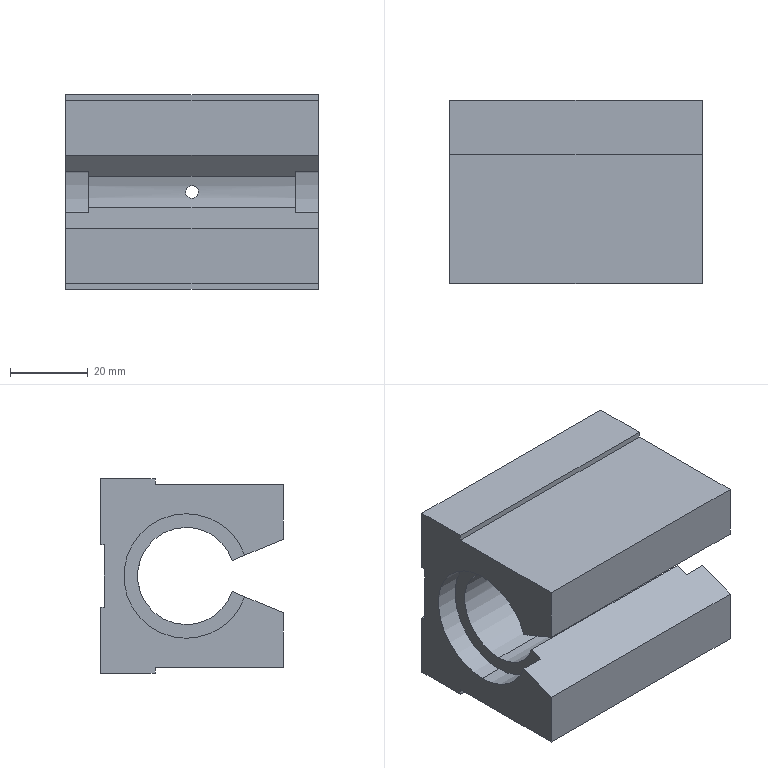Part | SolidWorks | features 3DProfileFeature 2, HoleWzd 2, ICE 2, Extrusion 1 | 1 solid | 46 faces | box 65 x 47 x 50 mm | volume 97950 mm3 | cylinder 19 | plane 19 | cone 8 | commonest cylinder face diameters 4.2 x8 32 x6 25 x3 3.3 x2
STEP:
#1=CARTESIAN_POINT('',(32.5,12.391,-1.65));
#2=VERTEX_POINT('',#1);
#3=CARTESIAN_POINT('',(32.5,12.391,1.65));
#4=VERTEX_POINT('',#3);
#5=CARTESIAN_POINT('',(32.5,12.391,-1.65));
#6=CARTESIAN_POINT('',(32.285,12.391,-1.65));
#7=CARTESIAN_POINT('',(32.067,12.397,-1.607));
#8=CARTESIAN_POINT('',(31.67,12.417,-1.442));
#9=CARTESIAN_POINT('',(31.486,12.431,-1.319));
#10=CARTESIAN_POINT('',(31.258,12.452,-1.092));
#11=CARTESIAN_POINT('',(31.188,12.46,-1.007));
#12=CARTESIAN_POINT('',(31.069,12.473,-0.8277));
#13=CARTESIAN_POINT('',(31.018,12.479,-0.733));
#14=CARTESIAN_POINT('',(30.935,12.489,-0.5333));
#15=CARTESIAN_POINT('',(30.903,12.493,-0.4285));
#16=CARTESIAN_POINT('',(30.861,12.499,-0.2176));
#17=CARTESIAN_POINT('',(30.85,12.5,-0.1102));
#18=CARTESIAN_POINT('',(30.85,12.5,0.1079));
#19=CARTESIAN_POINT('',(30.861,12.499,0.2152));
#20=CARTESIAN_POINT('',(30.902,12.493,0.4263));
#21=CARTESIAN_POINT('',(30.934,12.489,0.5312));
#22=CARTESIAN_POINT('',(31.017,12.479,0.7309));
#23=CARTESIAN_POINT('',(31.067,12.473,0.8257));
#24=CARTESIAN_POINT('',(31.187,12.46,1.005));
#25=CARTESIAN_POINT('',(31.257,12.453,1.09));
#26=CARTESIAN_POINT('',(31.484,12.431,1.318));
#27=CARTESIAN_POINT('',(31.668,12.417,1.441));
#28=CARTESIAN_POINT('',(32.065,12.397,1.606));
#29=CARTESIAN_POINT('',(32.282,12.391,1.65));
#30=CARTESIAN_POINT('',(32.5,12.391,1.65));
#31=B_SPLINE_CURVE_WITH_KNOTS('',3,(#5,#6,#7,#8,#9,#10,#11,#12,#13,#14,#15,#16,#17,#18,#19,#20,#21,#22,#23,#24,#25,#26,#27,#28,#29,#30),.UNSPECIFIED.,.F.,.F.,(4,2,2,2,2,2,2,2,2,2,2,2,4),(0.005164,0.00581,0.006455,0.006778,0.0071,0.007423,0.007746,0.008068,0.008391,0.008714,0.009037,0.009682,0.01033),.UNSPECIFIED.);
#32=EDGE_CURVE('',#2,#4,#31,.T.);
#33=ORIENTED_EDGE('',*,*,#32,.F.);
#34=CARTESIAN_POINT('',(32.5,21.,-1.65));
#35=VERTEX_POINT('',#34);
#36=CARTESIAN_POINT('',(32.5,22.,-1.65));
#37=DIRECTION('',(0.,1.,0.));
#38=VECTOR('',#37,1000.);
#39=LINE('',#36,#38);
#40=EDGE_CURVE('',#2,#35,#39,.T.);
#41=ORIENTED_EDGE('',*,*,#40,.T.);
#42=CARTESIAN_POINT('',(32.5,21.,1.65));
#43=VERTEX_POINT('',#42);
#44=CARTESIAN_POINT('',(32.5,21.,0.));
#45=DIRECTION('',(0.,-1.,0.));
#46=DIRECTION('',(0.,0.,-1.));
#47=AXIS2_PLACEMENT_3D('',#44,#45,#46);
#48=CIRCLE('',#47,1.65);
#49=EDGE_CURVE('',#43,#35,#48,.T.);
#50=ORIENTED_EDGE('',*,*,#49,.F.);
#51=CARTESIAN_POINT('',(32.5,22.,1.65));
#52=DIRECTION('',(0.,1.,0.));
#53=VECTOR('',#52,1000.);
#54=LINE('',#51,#53);
#55=EDGE_CURVE('',#4,#43,#54,.T.);
#56=ORIENTED_EDGE('',*,*,#55,.F.);
#57=EDGE_LOOP('',(#33,#41,#50,#56));
#58=FACE_OUTER_BOUND('',#57,.T.);
#59=CARTESIAN_POINT('',(32.5,22.,0.));
#60=DIRECTION('',(0.,1.,0.));
#61=DIRECTION('',(0.,0.,1.));
#62=AXIS2_PLACEMENT_3D('',#59,#60,#61);
#63=CYLINDRICAL_SURFACE('',#62,1.65);
#64=ADVANCED_FACE('',(#58),#63,.F.);
#65=CARTESIAN_POINT('',(12.5,9.6,-22.1));
#66=VERTEX_POINT('',#65);
#67=CARTESIAN_POINT('',(12.5,9.6,-17.9));
#68=VERTEX_POINT('',#67);
#69=CARTESIAN_POINT('',(12.5,9.6,-20.));
#70=DIRECTION('',(0.,1.,0.));
#71=DIRECTION('',(0.,0.,1.));
#72=AXIS2_PLACEMENT_3D('',#69,#70,#71);
#73=CIRCLE('',#72,2.1);
#74=EDGE_CURVE('',#66,#68,#73,.T.);
#75=ORIENTED_EDGE('',*,*,#74,.F.);
#76=CARTESIAN_POINT('',(12.5,22.,-22.1));
#77=VERTEX_POINT('',#76);
#78=CARTESIAN_POINT('',(12.5,22.,-22.1));
#79=DIRECTION('',(0.,1.,0.));
#80=VECTOR('',#79,1000.);
#81=LINE('',#78,#80);
#82=EDGE_CURVE('',#66,#77,#81,.T.);
#83=ORIENTED_EDGE('',*,*,#82,.T.);
#84=CARTESIAN_POINT('',(12.5,22.,-17.9));
#85=VERTEX_POINT('',#84);
#86=CARTESIAN_POINT('',(12.5,22.,-20.));
#87=DIRECTION('',(0.,1.,0.));
#88=DIRECTION('',(0.,0.,1.));
#89=AXIS2_PLACEMENT_3D('',#86,#87,#88);
#90=CIRCLE('',#89,2.1);
#91=EDGE_CURVE('',#77,#85,#90,.T.);
#92=ORIENTED_EDGE('',*,*,#91,.T.);
#93=CARTESIAN_POINT('',(12.5,22.,-17.9));
#94=DIRECTION('',(0.,1.,0.));
#95=VECTOR('',#94,1000.);
#96=LINE('',#93,#95);
#97=EDGE_CURVE('',#68,#85,#96,.T.);
#98=ORIENTED_EDGE('',*,*,#97,.F.);
#99=EDGE_LOOP('',(#75,#83,#92,#98));
#100=FACE_OUTER_BOUND('',#99,.T.);
#101=CARTESIAN_POINT('',(12.5,22.,-20.));
#102=DIRECTION('',(0.,1.,0.));
#103=DIRECTION('',(0.,0.,1.));
#104=AXIS2_PLACEMENT_3D('',#101,#102,#103);
#105=CYLINDRICAL_SURFACE('',#104,2.1);
#106=ADVANCED_FACE('',(#100),#105,.F.);
#107=CARTESIAN_POINT('',(12.5,8.338,-20.));
#108=VERTEX_POINT('',#107);
#109=CARTESIAN_POINT('',(12.5,9.6,-17.9));
#110=DIRECTION('',(0.,0.515,0.8572));
#111=VECTOR('',#110,1000.);
#112=LINE('',#109,#111);
#113=EDGE_CURVE('',#108,#68,#112,.T.);
#114=ORIENTED_EDGE('',*,*,#113,.F.);
#115=CARTESIAN_POINT('',(12.5,9.6,-22.1));
#116=DIRECTION('',(0.,0.515,-0.8572));
#117=VECTOR('',#116,1000.);
#118=LINE('',#115,#117);
#119=EDGE_CURVE('',#108,#66,#118,.T.);
#120=ORIENTED_EDGE('',*,*,#119,.T.);
#121=ORIENTED_EDGE('',*,*,#74,.T.);
#122=EDGE_LOOP('',(#114,#120,#121));
#123=FACE_OUTER_BOUND('',#122,.T.);
#124=CARTESIAN_POINT('',(12.5,9.6,-20.));
#125=DIRECTION('',(0.,1.,0.));
#126=DIRECTION('',(0.,0.,1.));
#127=AXIS2_PLACEMENT_3D('',#124,#125,#126);
#128=CONICAL_SURFACE('',#127,2.1,1.03);
#129=ADVANCED_FACE('',(#123),#128,.F.);
#130=CARTESIAN_POINT('',(52.5,9.6,-22.1));
#131=VERTEX_POINT('',#130);
#132=CARTESIAN_POINT('',(52.5,9.6,-17.9));
#133=VERTEX_POINT('',#132);
#134=CARTESIAN_POINT('',(52.5,9.6,-20.));
#135=DIRECTION('',(0.,1.,0.));
#136=DIRECTION('',(0.,0.,1.));
#137=AXIS2_PLACEMENT_3D('',#134,#135,#136);
#138=CIRCLE('',#137,2.1);
#139=EDGE_CURVE('',#131,#133,#138,.T.);
#140=ORIENTED_EDGE('',*,*,#139,.F.);
#141=CARTESIAN_POINT('',(52.5,22.,-22.1));
#142=VERTEX_POINT('',#141);
#143=CARTESIAN_POINT('',(52.5,22.,-22.1));
#144=DIRECTION('',(0.,1.,0.));
#145=VECTOR('',#144,1000.);
#146=LINE('',#143,#145);
#147=EDGE_CURVE('',#131,#142,#146,.T.);
#148=ORIENTED_EDGE('',*,*,#147,.T.);
#149=CARTESIAN_POINT('',(52.5,22.,-17.9));
#150=VERTEX_POINT('',#149);
#151=CARTESIAN_POINT('',(52.5,22.,-20.));
#152=DIRECTION('',(0.,1.,0.));
#153=DIRECTION('',(0.,0.,1.));
#154=AXIS2_PLACEMENT_3D('',#151,#152,#153);
#155=CIRCLE('',#154,2.1);
#156=EDGE_CURVE('',#142,#150,#155,.T.);
#157=ORIENTED_EDGE('',*,*,#156,.T.);
#158=CARTESIAN_POINT('',(52.5,22.,-17.9));
#159=DIRECTION('',(0.,1.,0.));
#160=VECTOR('',#159,1000.);
#161=LINE('',#158,#160);
#162=EDGE_CURVE('',#133,#150,#161,.T.);
#163=ORIENTED_EDGE('',*,*,#162,.F.);
#164=EDGE_LOOP('',(#140,#148,#157,#163));
#165=FACE_OUTER_BOUND('',#164,.T.);
#166=CARTESIAN_POINT('',(52.5,22.,-20.));
#167=DIRECTION('',(0.,1.,0.));
#168=DIRECTION('',(0.,0.,1.));
#169=AXIS2_PLACEMENT_3D('',#166,#167,#168);
#170=CYLINDRICAL_SURFACE('',#169,2.1);
#171=ADVANCED_FACE('',(#165),#170,.F.);
#172=CARTESIAN_POINT('',(52.5,8.338,-20.));
#173=VERTEX_POINT('',#172);
#174=CARTESIAN_POINT('',(52.5,9.6,-17.9));
#175=DIRECTION('',(0.,0.515,0.8572));
#176=VECTOR('',#175,1000.);
#177=LINE('',#174,#176);
#178=EDGE_CURVE('',#173,#133,#177,.T.);
#179=ORIENTED_EDGE('',*,*,#178,.F.);
#180=CARTESIAN_POINT('',(52.5,9.6,-22.1));
#181=DIRECTION('',(0.,0.515,-0.8572));
#182=VECTOR('',#181,1000.);
#183=LINE('',#180,#182);
#184=EDGE_CURVE('',#173,#131,#183,.T.);
#185=ORIENTED_EDGE('',*,*,#184,.T.);
#186=ORIENTED_EDGE('',*,*,#139,.T.);
#187=EDGE_LOOP('',(#179,#185,#186));
#188=FACE_OUTER_BOUND('',#187,.T.);
#189=CARTESIAN_POINT('',(52.5,9.6,-20.));
#190=DIRECTION('',(0.,1.,0.));
#191=DIRECTION('',(0.,0.,1.));
#192=AXIS2_PLACEMENT_3D('',#189,#190,#191);
#193=CONICAL_SURFACE('',#192,2.1,1.03);
#194=ADVANCED_FACE('',(#188),#193,.F.);
#195=CARTESIAN_POINT('',(12.5,9.6,17.9));
#196=VERTEX_POINT('',#195);
#197=CARTESIAN_POINT('',(12.5,9.6,22.1));
#198=VERTEX_POINT('',#197);
#199=CARTESIAN_POINT('',(12.5,9.6,20.));
#200=DIRECTION('',(0.,1.,0.));
#201=DIRECTION('',(0.,0.,1.));
#202=AXIS2_PLACEMENT_3D('',#199,#200,#201);
#203=CIRCLE('',#202,2.1);
#204=EDGE_CURVE('',#196,#198,#203,.T.);
#205=ORIENTED_EDGE('',*,*,#204,.F.);
#206=CARTESIAN_POINT('',(12.5,22.,17.9));
#207=VERTEX_POINT('',#206);
#208=CARTESIAN_POINT('',(12.5,22.,17.9));
#209=DIRECTION('',(0.,1.,0.));
#210=VECTOR('',#209,1000.);
#211=LINE('',#208,#210);
#212=EDGE_CURVE('',#196,#207,#211,.T.);
#213=ORIENTED_EDGE('',*,*,#212,.T.);
#214=CARTESIAN_POINT('',(12.5,22.,22.1));
#215=VERTEX_POINT('',#214);
#216=CARTESIAN_POINT('',(12.5,22.,20.));
#217=DIRECTION('',(0.,1.,0.));
#218=DIRECTION('',(0.,0.,1.));
#219=AXIS2_PLACEMENT_3D('',#216,#217,#218);
#220=CIRCLE('',#219,2.1);
#221=EDGE_CURVE('',#207,#215,#220,.T.);
#222=ORIENTED_EDGE('',*,*,#221,.T.);
#223=CARTESIAN_POINT('',(12.5,22.,22.1));
#224=DIRECTION('',(0.,1.,0.));
#225=VECTOR('',#224,1000.);
#226=LINE('',#223,#225);
#227=EDGE_CURVE('',#198,#215,#226,.T.);
#228=ORIENTED_EDGE('',*,*,#227,.F.);
#229=EDGE_LOOP('',(#205,#213,#222,#228));
#230=FACE_OUTER_BOUND('',#229,.T.);
#231=CARTESIAN_POINT('',(12.5,22.,20.));
#232=DIRECTION('',(0.,1.,0.));
#233=DIRECTION('',(0.,0.,1.));
#234=AXIS2_PLACEMENT_3D('',#231,#232,#233);
#235=CYLINDRICAL_SURFACE('',#234,2.1);
#236=ADVANCED_FACE('',(#230),#235,.F.);
#237=CARTESIAN_POINT('',(12.5,8.338,20.));
#238=VERTEX_POINT('',#237);
#239=CARTESIAN_POINT('',(12.5,9.6,22.1));
#240=DIRECTION('',(0.,0.515,0.8572));
#241=VECTOR('',#240,1000.);
#242=LINE('',#239,#241);
#243=EDGE_CURVE('',#238,#198,#242,.T.);
#244=ORIENTED_EDGE('',*,*,#243,.F.);
#245=CARTESIAN_POINT('',(12.5,9.6,17.9));
#246=DIRECTION('',(0.,0.515,-0.8572));
#247=VECTOR('',#246,1000.);
#248=LINE('',#245,#247);
#249=EDGE_CURVE('',#238,#196,#248,.T.);
#250=ORIENTED_EDGE('',*,*,#249,.T.);
#251=ORIENTED_EDGE('',*,*,#204,.T.);
#252=EDGE_LOOP('',(#244,#250,#251));
#253=FACE_OUTER_BOUND('',#252,.T.);
#254=CARTESIAN_POINT('',(12.5,9.6,20.));
#255=DIRECTION('',(0.,1.,0.));
#256=DIRECTION('',(0.,0.,1.));
#257=AXIS2_PLACEMENT_3D('',#254,#255,#256);
#258=CONICAL_SURFACE('',#257,2.1,1.03);
#259=ADVANCED_FACE('',(#253),#258,.F.);
#260=CARTESIAN_POINT('',(52.5,9.6,17.9));
#261=VERTEX_POINT('',#260);
#262=CARTESIAN_POINT('',(52.5,9.6,22.1));
#263=VERTEX_POINT('',#262);
#264=CARTESIAN_POINT('',(52.5,9.6,20.));
#265=DIRECTION('',(0.,1.,0.));
#266=DIRECTION('',(0.,0.,1.));
#267=AXIS2_PLACEMENT_3D('',#264,#265,#266);
#268=CIRCLE('',#267,2.1);
#269=EDGE_CURVE('',#261,#263,#268,.T.);
#270=ORIENTED_EDGE('',*,*,#269,.F.);
#271=CARTESIAN_POINT('',(52.5,22.,17.9));
#272=VERTEX_POINT('',#271);
#273=CARTESIAN_POINT('',(52.5,22.,17.9));
#274=DIRECTION('',(0.,1.,0.));
#275=VECTOR('',#274,1000.);
#276=LINE('',#273,#275);
#277=EDGE_CURVE('',#261,#272,#276,.T.);
#278=ORIENTED_EDGE('',*,*,#277,.T.);
#279=CARTESIAN_POINT('',(52.5,22.,22.1));
#280=VERTEX_POINT('',#279);
#281=CARTESIAN_POINT('',(52.5,22.,20.));
#282=DIRECTION('',(0.,1.,0.));
#283=DIRECTION('',(0.,0.,1.));
#284=AXIS2_PLACEMENT_3D('',#281,#282,#283);
#285=CIRCLE('',#284,2.1);
#286=EDGE_CURVE('',#272,#280,#285,.T.);
#287=ORIENTED_EDGE('',*,*,#286,.T.);
#288=CARTESIAN_POINT('',(52.5,22.,22.1));
#289=DIRECTION('',(0.,1.,0.));
#290=VECTOR('',#289,1000.);
#291=LINE('',#288,#290);
#292=EDGE_CURVE('',#263,#280,#291,.T.);
#293=ORIENTED_EDGE('',*,*,#292,.F.);
#294=EDGE_LOOP('',(#270,#278,#287,#293));
#295=FACE_OUTER_BOUND('',#294,.T.);
#296=CARTESIAN_POINT('',(52.5,22.,20.));
#297=DIRECTION('',(0.,1.,0.));
#298=DIRECTION('',(0.,0.,1.));
#299=AXIS2_PLACEMENT_3D('',#296,#297,#298);
#300=CYLINDRICAL_SURFACE('',#299,2.1);
#301=ADVANCED_FACE('',(#295),#300,.F.);
#302=CARTESIAN_POINT('',(52.5,8.338,20.));
#303=VERTEX_POINT('',#302);
#304=CARTESIAN_POINT('',(52.5,9.6,22.1));
#305=DIRECTION('',(0.,0.515,0.8572));
#306=VECTOR('',#305,1000.);
#307=LINE('',#304,#306);
#308=EDGE_CURVE('',#303,#263,#307,.T.);
#309=ORIENTED_EDGE('',*,*,#308,.F.);
#310=CARTESIAN_POINT('',(52.5,9.6,17.9));
#311=DIRECTION('',(0.,0.515,-0.8572));
#312=VECTOR('',#311,1000.);
#313=LINE('',#310,#312);
#314=EDGE_CURVE('',#303,#261,#313,.T.);
#315=ORIENTED_EDGE('',*,*,#314,.T.);
#316=ORIENTED_EDGE('',*,*,#269,.T.);
#317=EDGE_LOOP('',(#309,#315,#316));
#318=FACE_OUTER_BOUND('',#317,.T.);
#319=CARTESIAN_POINT('',(52.5,9.6,20.));
#320=DIRECTION('',(0.,1.,0.));
#321=DIRECTION('',(0.,0.,1.));
#322=AXIS2_PLACEMENT_3D('',#319,#320,#321);
#323=CONICAL_SURFACE('',#322,2.1,1.03);
#324=ADVANCED_FACE('',(#318),#323,.F.);
#325=CARTESIAN_POINT('',(6.,0.,-16.));
#326=VERTEX_POINT('',#325);
#327=CARTESIAN_POINT('',(6.,-15.082,-5.342));
#328=VERTEX_POINT('',#327);
#329=CARTESIAN_POINT('',(6.,0.,0.));
#330=DIRECTION('',(-1.,0.,0.));
#331=DIRECTION('',(0.,0.,1.));
#332=AXIS2_PLACEMENT_3D('',#329,#330,#331);
#333=CIRCLE('',#332,16.);
#334=EDGE_CURVE('',#326,#328,#333,.T.);
#335=ORIENTED_EDGE('',*,*,#334,.F.);
#336=CARTESIAN_POINT('',(0.,0.,-16.));
#337=VERTEX_POINT('',#336);
#338=CARTESIAN_POINT('',(6.,0.,-16.));
#339=DIRECTION('',(-1.,0.,0.));
#340=VECTOR('',#339,1000.);
#341=LINE('',#338,#340);
#342=EDGE_CURVE('',#326,#337,#341,.T.);
#343=ORIENTED_EDGE('',*,*,#342,.T.);
#344=CARTESIAN_POINT('',(0.,-15.082,-5.342));
#345=VERTEX_POINT('',#344);
#346=CARTESIAN_POINT('',(0.,0.,0.));
#347=DIRECTION('',(1.,0.,0.));
#348=DIRECTION('',(0.,0.,-1.));
#349=AXIS2_PLACEMENT_3D('',#346,#347,#348);
#350=CIRCLE('',#349,16.);
#351=EDGE_CURVE('',#345,#337,#350,.T.);
#352=ORIENTED_EDGE('',*,*,#351,.F.);
#353=CARTESIAN_POINT('',(6.,-15.082,-5.342));
#354=DIRECTION('',(-1.,0.,0.));
#355=VECTOR('',#354,1000.);
#356=LINE('',#353,#355);
#357=EDGE_CURVE('',#328,#345,#356,.T.);
#358=ORIENTED_EDGE('',*,*,#357,.F.);
#359=EDGE_LOOP('',(#335,#343,#352,#358));
#360=FACE_OUTER_BOUND('',#359,.T.);
#361=CARTESIAN_POINT('',(6.,0.,0.));
#362=DIRECTION('',(-1.,0.,0.));
#363=DIRECTION('',(0.,0.,1.));
#364=AXIS2_PLACEMENT_3D('',#361,#362,#363);
#365=CYLINDRICAL_SURFACE('',#364,16.);
#366=ADVANCED_FACE('',(#360),#365,.F.);
#367=ORIENTED_EDGE('',*,*,#342,.F.);
#368=CARTESIAN_POINT('',(6.,0.,16.));
#369=VERTEX_POINT('',#368);
#370=CARTESIAN_POINT('',(6.,0.,0.));
#371=DIRECTION('',(-1.,0.,0.));
#372=DIRECTION('',(0.,0.,1.));
#373=AXIS2_PLACEMENT_3D('',#370,#371,#372);
#374=CIRCLE('',#373,16.);
#375=EDGE_CURVE('',#369,#326,#374,.T.);
#376=ORIENTED_EDGE('',*,*,#375,.F.);
#377=CARTESIAN_POINT('',(0.,0.,16.));
#378=VERTEX_POINT('',#377);
#379=CARTESIAN_POINT('',(6.,0.,16.));
#380=DIRECTION('',(-1.,0.,0.));
#381=VECTOR('',#380,1000.);
#382=LINE('',#379,#381);
#383=EDGE_CURVE('',#369,#378,#382,.T.);
#384=ORIENTED_EDGE('',*,*,#383,.T.);
#385=CARTESIAN_POINT('',(0.,0.,0.));
#386=DIRECTION('',(1.,0.,0.));
#387=DIRECTION('',(0.,0.,-1.));
#388=AXIS2_PLACEMENT_3D('',#385,#386,#387);
#389=CIRCLE('',#388,16.);
#390=EDGE_CURVE('',#337,#378,#389,.T.);
#391=ORIENTED_EDGE('',*,*,#390,.F.);
#392=EDGE_LOOP('',(#367,#376,#384,#391));
#393=FACE_OUTER_BOUND('',#392,.T.);
#394=CARTESIAN_POINT('',(6.,0.,0.));
#395=DIRECTION('',(-1.,0.,0.));
#396=DIRECTION('',(0.,0.,1.));
#397=AXIS2_PLACEMENT_3D('',#394,#395,#396);
#398=CYLINDRICAL_SURFACE('',#397,16.);
#399=ADVANCED_FACE('',(#393),#398,.F.);
#400=CARTESIAN_POINT('',(59.,0.,16.));
#401=VERTEX_POINT('',#400);
#402=CARTESIAN_POINT('',(59.,-15.082,5.342));
#403=VERTEX_POINT('',#402);
#404=CARTESIAN_POINT('',(59.,0.,0.));
#405=DIRECTION('',(1.,0.,0.));
#406=DIRECTION('',(0.,0.,-1.));
#407=AXIS2_PLACEMENT_3D('',#404,#405,#406);
#408=CIRCLE('',#407,16.);
#409=EDGE_CURVE('',#401,#403,#408,.T.);
#410=ORIENTED_EDGE('',*,*,#409,.F.);
#411=CARTESIAN_POINT('',(65.,0.,16.));
#412=VERTEX_POINT('',#411);
#413=CARTESIAN_POINT('',(59.,0.,16.));
#414=DIRECTION('',(1.,0.,0.));
#415=VECTOR('',#414,1000.);
#416=LINE('',#413,#415);
#417=EDGE_CURVE('',#401,#412,#416,.T.);
#418=ORIENTED_EDGE('',*,*,#417,.T.);
#419=CARTESIAN_POINT('',(65.,-15.082,5.342));
#420=VERTEX_POINT('',#419);
#421=CARTESIAN_POINT('',(65.,0.,0.));
#422=DIRECTION('',(1.,0.,0.));
#423=DIRECTION('',(0.,0.,-1.));
#424=AXIS2_PLACEMENT_3D('',#421,#422,#423);
#425=CIRCLE('',#424,16.);
#426=EDGE_CURVE('',#412,#420,#425,.T.);
#427=ORIENTED_EDGE('',*,*,#426,.T.);
#428=CARTESIAN_POINT('',(59.,-15.082,5.342));
#429=DIRECTION('',(1.,0.,0.));
#430=VECTOR('',#429,1000.);
#431=LINE('',#428,#430);
#432=EDGE_CURVE('',#403,#420,#431,.T.);
#433=ORIENTED_EDGE('',*,*,#432,.F.);
#434=EDGE_LOOP('',(#410,#418,#427,#433));
#435=FACE_OUTER_BOUND('',#434,.T.);
#436=CARTESIAN_POINT('',(59.,0.,0.));
#437=DIRECTION('',(1.,0.,0.));
#438=DIRECTION('',(0.,0.,-1.));
#439=AXIS2_PLACEMENT_3D('',#436,#437,#438);
#440=CYLINDRICAL_SURFACE('',#439,16.);
#441=ADVANCED_FACE('',(#435),#440,.F.);
#442=ORIENTED_EDGE('',*,*,#417,.F.);
#443=CARTESIAN_POINT('',(59.,0.,-16.));
#444=VERTEX_POINT('',#443);
#445=CARTESIAN_POINT('',(59.,0.,0.));
#446=DIRECTION('',(1.,0.,0.));
#447=DIRECTION('',(0.,0.,-1.));
#448=AXIS2_PLACEMENT_3D('',#445,#446,#447);
#449=CIRCLE('',#448,16.);
#450=EDGE_CURVE('',#444,#401,#449,.T.);
#451=ORIENTED_EDGE('',*,*,#450,.F.);
#452=CARTESIAN_POINT('',(65.,0.,-16.));
#453=VERTEX_POINT('',#452);
#454=CARTESIAN_POINT('',(59.,0.,-16.));
#455=DIRECTION('',(1.,0.,0.));
#456=VECTOR('',#455,1000.);
#457=LINE('',#454,#456);
#458=EDGE_CURVE('',#444,#453,#457,.T.);
#459=ORIENTED_EDGE('',*,*,#458,.T.);
#460=CARTESIAN_POINT('',(65.,0.,0.));
#461=DIRECTION('',(1.,0.,0.));
#462=DIRECTION('',(0.,0.,-1.));
#463=AXIS2_PLACEMENT_3D('',#460,#461,#462);
#464=CIRCLE('',#463,16.);
#465=EDGE_CURVE('',#453,#412,#464,.T.);
#466=ORIENTED_EDGE('',*,*,#465,.T.);
#467=EDGE_LOOP('',(#442,#451,#459,#466));
#468=FACE_OUTER_BOUND('',#467,.T.);
#469=CARTESIAN_POINT('',(59.,0.,0.));
#470=DIRECTION('',(1.,0.,0.));
#471=DIRECTION('',(0.,0.,-1.));
#472=AXIS2_PLACEMENT_3D('',#469,#470,#471);
#473=CYLINDRICAL_SURFACE('',#472,16.);
#474=ADVANCED_FACE('',(#468),#473,.F.);
#475=CARTESIAN_POINT('',(59.,0.,-12.5));
#476=VERTEX_POINT('',#475);
#477=CARTESIAN_POINT('',(59.,-11.843,-4.));
#478=VERTEX_POINT('',#477);
#479=CARTESIAN_POINT('',(59.,0.,0.));
#480=DIRECTION('',(-1.,0.,0.));
#481=DIRECTION('',(0.,0.,-1.));
#482=AXIS2_PLACEMENT_3D('',#479,#480,#481);
#483=CIRCLE('',#482,12.5);
#484=EDGE_CURVE('',#476,#478,#483,.T.);
#485=ORIENTED_EDGE('',*,*,#484,.F.);
#486=CARTESIAN_POINT('',(6.,0.,-12.5));
#487=VERTEX_POINT('',#486);
#488=CARTESIAN_POINT('',(65.,0.,-12.5));
#489=DIRECTION('',(-1.,0.,0.));
#490=VECTOR('',#489,1000.);
#491=LINE('',#488,#490);
#492=EDGE_CURVE('',#476,#487,#491,.T.);
#493=ORIENTED_EDGE('',*,*,#492,.T.);
#494=CARTESIAN_POINT('',(6.,-11.843,-4.));
#495=VERTEX_POINT('',#494);
#496=CARTESIAN_POINT('',(6.,0.,0.));
#497=DIRECTION('',(1.,0.,0.));
#498=DIRECTION('',(0.,0.,1.));
#499=AXIS2_PLACEMENT_3D('',#496,#497,#498);
#500=CIRCLE('',#499,12.5);
#501=EDGE_CURVE('',#495,#487,#500,.T.);
#502=ORIENTED_EDGE('',*,*,#501,.F.);
#503=CARTESIAN_POINT('',(65.,-11.843,-4.));
#504=DIRECTION('',(-1.,0.,0.));
#505=VECTOR('',#504,1000.);
#506=LINE('',#503,#505);
#507=EDGE_CURVE('',#478,#495,#506,.T.);
#508=ORIENTED_EDGE('',*,*,#507,.F.);
#509=EDGE_LOOP('',(#485,#493,#502,#508));
#510=FACE_OUTER_BOUND('',#509,.T.);
#511=CARTESIAN_POINT('',(65.,0.,0.));
#512=DIRECTION('',(-1.,0.,0.));
#513=DIRECTION('',(0.,0.,1.));
#514=AXIS2_PLACEMENT_3D('',#511,#512,#513);
#515=CYLINDRICAL_SURFACE('',#514,12.5);
#516=ADVANCED_FACE('',(#510),#515,.F.);
#517=ORIENTED_EDGE('',*,*,#492,.F.);
#518=CARTESIAN_POINT('',(59.,0.,12.5));
#519=VERTEX_POINT('',#518);
#520=CARTESIAN_POINT('',(59.,0.,0.));
#521=DIRECTION('',(-1.,0.,0.));
#522=DIRECTION('',(0.,0.,-1.));
#523=AXIS2_PLACEMENT_3D('',#520,#521,#522);
#524=CIRCLE('',#523,12.5);
#525=EDGE_CURVE('',#519,#476,#524,.T.);
#526=ORIENTED_EDGE('',*,*,#525,.F.);
#527=CARTESIAN_POINT('',(6.,0.,12.5));
#528=VERTEX_POINT('',#527);
#529=CARTESIAN_POINT('',(65.,0.,12.5));
#530=DIRECTION('',(-1.,0.,0.));
#531=VECTOR('',#530,1000.);
#532=LINE('',#529,#531);
#533=EDGE_CURVE('',#519,#528,#532,.T.);
#534=ORIENTED_EDGE('',*,*,#533,.T.);
#535=CARTESIAN_POINT('',(6.,0.,0.));
#536=DIRECTION('',(1.,0.,0.));
#537=DIRECTION('',(0.,0.,1.));
#538=AXIS2_PLACEMENT_3D('',#535,#536,#537);
#539=CIRCLE('',#538,12.5);
#540=EDGE_CURVE('',#487,#528,#539,.T.);
#541=ORIENTED_EDGE('',*,*,#540,.F.);
#542=EDGE_LOOP('',(#517,#526,#534,#541));
#543=FACE_OUTER_BOUND('',#542,.T.);
#544=CARTESIAN_POINT('',(32.5,12.391,1.65));
#545=CARTESIAN_POINT('',(32.609,12.391,1.65));
#546=CARTESIAN_POINT('',(32.716,12.392,1.639));
#547=CARTESIAN_POINT('',(32.928,12.398,1.597));
#548=CARTESIAN_POINT('',(33.032,12.402,1.565));
#549=CARTESIAN_POINT('',(33.232,12.412,1.483));
#550=CARTESIAN_POINT('',(33.327,12.418,1.432));
#551=CARTESIAN_POINT('',(33.506,12.431,1.312));
#552=CARTESIAN_POINT('',(33.591,12.438,1.243));
#553=CARTESIAN_POINT('',(33.819,12.46,1.014));
#554=CARTESIAN_POINT('',(33.942,12.474,0.8305));
#555=CARTESIAN_POINT('',(34.106,12.494,0.4334));
#556=CARTESIAN_POINT('',(34.15,12.5,0.2161));
#557=CARTESIAN_POINT('',(34.15,12.5,-0.1071));
#558=CARTESIAN_POINT('',(34.139,12.499,-0.2166));
#559=CARTESIAN_POINT('',(34.097,12.493,-0.4283));
#560=CARTESIAN_POINT('',(34.066,12.489,-0.5312));
#561=CARTESIAN_POINT('',(33.983,12.479,-0.7312));
#562=CARTESIAN_POINT('',(33.931,12.473,-0.8276));
#563=CARTESIAN_POINT('',(33.812,12.46,-1.006));
#564=CARTESIAN_POINT('',(33.744,12.453,-1.09));
#565=CARTESIAN_POINT('',(33.59,12.438,-1.244));
#566=CARTESIAN_POINT('',(33.507,12.431,-1.312));
#567=CARTESIAN_POINT('',(33.328,12.418,-1.431));
#568=CARTESIAN_POINT('',(33.232,12.412,-1.483));
#569=CARTESIAN_POINT('',(33.032,12.402,-1.566));
#570=CARTESIAN_POINT('',(32.929,12.398,-1.597));
#571=CARTESIAN_POINT('',(32.717,12.392,-1.639));
#572=CARTESIAN_POINT('',(32.608,12.391,-1.65));
#573=CARTESIAN_POINT('',(32.5,12.391,-1.65));
#574=B_SPLINE_CURVE_WITH_KNOTS('',3,(#544,#545,#546,#547,#548,#549,#550,#551,#552,#553,#554,#555,#556,#557,#558,#559,#560,#561,#562,#563,#564,#565,#566,#567,#568,#569,#570,#571,#572,#573),.UNSPECIFIED.,.F.,.F.,(4,2,2,2,2,2,2,2,2,2,2,2,2,2,4),(0.,0.0003228,0.0006455,0.0009683,0.001291,0.001937,0.002582,0.002905,0.003228,0.00355,0.003873,0.004196,0.004519,0.004842,0.005164),.UNSPECIFIED.);
#575=EDGE_CURVE('',#4,#2,#574,.T.);
#576=ORIENTED_EDGE('',*,*,#575,.T.);
#577=ORIENTED_EDGE('',*,*,#32,.T.);
#578=EDGE_LOOP('',(#576,#577));
#579=FACE_BOUND('',#578,.T.);
#580=CARTESIAN_POINT('',(65.,0.,0.));
#581=DIRECTION('',(-1.,0.,0.));
#582=DIRECTION('',(0.,0.,1.));
#583=AXIS2_PLACEMENT_3D('',#580,#581,#582);
#584=CYLINDRICAL_SURFACE('',#583,12.5);
#585=ADVANCED_FACE('',(#543,#579),#584,.F.);
#586=ORIENTED_EDGE('',*,*,#533,.F.);
#587=CARTESIAN_POINT('',(59.,-11.843,4.));
#588=VERTEX_POINT('',#587);
#589=CARTESIAN_POINT('',(59.,0.,0.));
#590=DIRECTION('',(-1.,0.,0.));
#591=DIRECTION('',(0.,0.,-1.));
#592=AXIS2_PLACEMENT_3D('',#589,#590,#591);
#593=CIRCLE('',#592,12.5);
#594=EDGE_CURVE('',#588,#519,#593,.T.);
#595=ORIENTED_EDGE('',*,*,#594,.F.);
#596=CARTESIAN_POINT('',(6.,-11.843,4.));
#597=VERTEX_POINT('',#596);
#598=CARTESIAN_POINT('',(65.,-11.843,4.));
#599=DIRECTION('',(-1.,0.,0.));
#600=VECTOR('',#599,1000.);
#601=LINE('',#598,#600);
#602=EDGE_CURVE('',#588,#597,#601,.T.);
#603=ORIENTED_EDGE('',*,*,#602,.T.);
#604=CARTESIAN_POINT('',(6.,0.,0.));
#605=DIRECTION('',(1.,0.,0.));
#606=DIRECTION('',(0.,0.,1.));
#607=AXIS2_PLACEMENT_3D('',#604,#605,#606);
#608=CIRCLE('',#607,12.5);
#609=EDGE_CURVE('',#528,#597,#608,.T.);
#610=ORIENTED_EDGE('',*,*,#609,.F.);
#611=EDGE_LOOP('',(#586,#595,#603,#610));
#612=FACE_OUTER_BOUND('',#611,.T.);
#613=CARTESIAN_POINT('',(65.,0.,0.));
#614=DIRECTION('',(-1.,0.,0.));
#615=DIRECTION('',(0.,0.,1.));
#616=AXIS2_PLACEMENT_3D('',#613,#614,#615);
#617=CYLINDRICAL_SURFACE('',#616,12.5);
#618=ADVANCED_FACE('',(#612),#617,.F.);
#619=CARTESIAN_POINT('',(6.,-25.,-9.45));
#620=DIRECTION('',(0.,0.9239,0.3827));
#621=VECTOR('',#620,1000.);
#622=LINE('',#619,#621);
#623=EDGE_CURVE('',#328,#495,#622,.T.);
#624=ORIENTED_EDGE('',*,*,#623,.F.);
#625=ORIENTED_EDGE('',*,*,#357,.T.);
#626=CARTESIAN_POINT('',(0.,-25.,-9.45));
#627=VERTEX_POINT('',#626);
#628=CARTESIAN_POINT('',(0.,-25.,-9.45));
#629=DIRECTION('',(0.,-0.9239,-0.3827));
#630=VECTOR('',#629,1000.);
#631=LINE('',#628,#630);
#632=EDGE_CURVE('',#345,#627,#631,.T.);
#633=ORIENTED_EDGE('',*,*,#632,.T.);
#634=CARTESIAN_POINT('',(65.,-25.,-9.45));
#635=VERTEX_POINT('',#634);
#636=CARTESIAN_POINT('',(65.,-25.,-9.45));
#637=DIRECTION('',(-1.,0.,0.));
#638=VECTOR('',#637,1000.);
#639=LINE('',#636,#638);
#640=EDGE_CURVE('',#635,#627,#639,.T.);
#641=ORIENTED_EDGE('',*,*,#640,.F.);
#642=CARTESIAN_POINT('',(65.,-15.082,-5.342));
#643=VERTEX_POINT('',#642);
#644=CARTESIAN_POINT('',(65.,-25.,-9.45));
#645=DIRECTION('',(0.,-0.9239,-0.3827));
#646=VECTOR('',#645,1000.);
#647=LINE('',#644,#646);
#648=EDGE_CURVE('',#643,#635,#647,.T.);
#649=ORIENTED_EDGE('',*,*,#648,.F.);
#650=CARTESIAN_POINT('',(59.,-15.082,-5.342));
#651=VERTEX_POINT('',#650);
#652=CARTESIAN_POINT('',(59.,-15.082,-5.342));
#653=DIRECTION('',(-1.,0.,0.));
#654=VECTOR('',#653,1000.);
#655=LINE('',#652,#654);
#656=EDGE_CURVE('',#643,#651,#655,.T.);
#657=ORIENTED_EDGE('',*,*,#656,.T.);
#658=CARTESIAN_POINT('',(59.,-25.,-9.45));
#659=DIRECTION('',(0.,-0.9239,-0.3827));
#660=VECTOR('',#659,1000.);
#661=LINE('',#658,#660);
#662=EDGE_CURVE('',#478,#651,#661,.T.);
#663=ORIENTED_EDGE('',*,*,#662,.F.);
#664=ORIENTED_EDGE('',*,*,#507,.T.);
#665=EDGE_LOOP('',(#624,#625,#633,#641,#649,#657,#663,#664));
#666=FACE_OUTER_BOUND('',#665,.T.);
#667=CARTESIAN_POINT('',(65.,-25.,-9.45));
#668=DIRECTION('',(0.,0.3827,-0.9239));
#669=DIRECTION('',(0.,0.9239,0.3827));
#670=AXIS2_PLACEMENT_3D('',#667,#668,#669);
#671=PLANE('',#670);
#672=ADVANCED_FACE('',(#666),#671,.F.);
#673=CARTESIAN_POINT('',(0.,-25.,-23.5));
#674=VERTEX_POINT('',#673);
#675=CARTESIAN_POINT('',(0.,-25.,-9.45));
#676=DIRECTION('',(0.,0.,-1.));
#677=VECTOR('',#676,1000.);
#678=LINE('',#675,#677);
#679=EDGE_CURVE('',#627,#674,#678,.T.);
#680=ORIENTED_EDGE('',*,*,#679,.T.);
#681=CARTESIAN_POINT('',(65.,-25.,-23.5));
#682=VERTEX_POINT('',#681);
#683=CARTESIAN_POINT('',(65.,-25.,-23.5));
#684=DIRECTION('',(-1.,0.,0.));
#685=VECTOR('',#684,1000.);
#686=LINE('',#683,#685);
#687=EDGE_CURVE('',#682,#674,#686,.T.);
#688=ORIENTED_EDGE('',*,*,#687,.F.);
#689=CARTESIAN_POINT('',(65.,-25.,-9.45));
#690=DIRECTION('',(0.,0.,-1.));
#691=VECTOR('',#690,1000.);
#692=LINE('',#689,#691);
#693=EDGE_CURVE('',#635,#682,#692,.T.);
#694=ORIENTED_EDGE('',*,*,#693,.F.);
#695=ORIENTED_EDGE('',*,*,#640,.T.);
#696=EDGE_LOOP('',(#680,#688,#694,#695));
#697=FACE_OUTER_BOUND('',#696,.T.);
#698=CARTESIAN_POINT('',(65.,-25.,-9.45));
#699=DIRECTION('',(0.,1.,0.));
#700=DIRECTION('',(0.,0.,1.));
#701=AXIS2_PLACEMENT_3D('',#698,#699,#700);
#702=PLANE('',#701);
#703=ADVANCED_FACE('',(#697),#702,.F.);
#704=CARTESIAN_POINT('',(0.,8.,-23.5));
#705=VERTEX_POINT('',#704);
#706=CARTESIAN_POINT('',(0.,-25.,-23.5));
#707=DIRECTION('',(0.,1.,0.));
#708=VECTOR('',#707,1000.);
#709=LINE('',#706,#708);
#710=EDGE_CURVE('',#674,#705,#709,.T.);
#711=ORIENTED_EDGE('',*,*,#710,.T.);
#712=CARTESIAN_POINT('',(65.,8.,-23.5));
#713=VERTEX_POINT('',#712);
#714=CARTESIAN_POINT('',(65.,8.,-23.5));
#715=DIRECTION('',(-1.,0.,0.));
#716=VECTOR('',#715,1000.);
#717=LINE('',#714,#716);
#718=EDGE_CURVE('',#713,#705,#717,.T.);
#719=ORIENTED_EDGE('',*,*,#718,.F.);
#720=CARTESIAN_POINT('',(65.,-25.,-23.5));
#721=DIRECTION('',(0.,1.,0.));
#722=VECTOR('',#721,1000.);
#723=LINE('',#720,#722);
#724=EDGE_CURVE('',#682,#713,#723,.T.);
#725=ORIENTED_EDGE('',*,*,#724,.F.);
#726=ORIENTED_EDGE('',*,*,#687,.T.);
#727=EDGE_LOOP('',(#711,#719,#725,#726));
#728=FACE_OUTER_BOUND('',#727,.T.);
#729=CARTESIAN_POINT('',(65.,-25.,-23.5));
#730=DIRECTION('',(0.,0.,1.));
#731=DIRECTION('',(1.,0.,0.));
#732=AXIS2_PLACEMENT_3D('',#729,#730,#731);
#733=PLANE('',#732);
#734=ADVANCED_FACE('',(#728),#733,.F.);
#735=CARTESIAN_POINT('',(0.,8.,-25.));
#736=VERTEX_POINT('',#735);
#737=CARTESIAN_POINT('',(0.,8.,-23.5));
#738=DIRECTION('',(0.,0.,-1.));
#739=VECTOR('',#738,1000.);
#740=LINE('',#737,#739);
#741=EDGE_CURVE('',#705,#736,#740,.T.);
#742=ORIENTED_EDGE('',*,*,#741,.T.);
#743=CARTESIAN_POINT('',(65.,8.,-25.));
#744=VERTEX_POINT('',#743);
#745=CARTESIAN_POINT('',(65.,8.,-25.));
#746=DIRECTION('',(-1.,0.,0.));
#747=VECTOR('',#746,1000.);
#748=LINE('',#745,#747);
#749=EDGE_CURVE('',#744,#736,#748,.T.);
#750=ORIENTED_EDGE('',*,*,#749,.F.);
#751=CARTESIAN_POINT('',(65.,8.,-23.5));
#752=DIRECTION('',(0.,0.,-1.));
#753=VECTOR('',#752,1000.);
#754=LINE('',#751,#753);
#755=EDGE_CURVE('',#713,#744,#754,.T.);
#756=ORIENTED_EDGE('',*,*,#755,.F.);
#757=ORIENTED_EDGE('',*,*,#718,.T.);
#758=EDGE_LOOP('',(#742,#750,#756,#757));
#759=FACE_OUTER_BOUND('',#758,.T.);
#760=CARTESIAN_POINT('',(65.,8.,-23.5));
#761=DIRECTION('',(0.,1.,0.));
#762=DIRECTION('',(0.,0.,1.));
#763=AXIS2_PLACEMENT_3D('',#760,#761,#762);
#764=PLANE('',#763);
#765=ADVANCED_FACE('',(#759),#764,.F.);
#766=CARTESIAN_POINT('',(0.,22.,-25.));
#767=VERTEX_POINT('',#766);
#768=CARTESIAN_POINT('',(0.,8.,-25.));
#769=DIRECTION('',(0.,1.,0.));
#770=VECTOR('',#769,1000.);
#771=LINE('',#768,#770);
#772=EDGE_CURVE('',#736,#767,#771,.T.);
#773=ORIENTED_EDGE('',*,*,#772,.T.);
#774=CARTESIAN_POINT('',(65.,22.,-25.));
#775=VERTEX_POINT('',#774);
#776=CARTESIAN_POINT('',(65.,22.,-25.));
#777=DIRECTION('',(-1.,0.,0.));
#778=VECTOR('',#777,1000.);
#779=LINE('',#776,#778);
#780=EDGE_CURVE('',#775,#767,#779,.T.);
#781=ORIENTED_EDGE('',*,*,#780,.F.);
#782=CARTESIAN_POINT('',(65.,8.,-25.));
#783=DIRECTION('',(0.,1.,0.));
#784=VECTOR('',#783,1000.);
#785=LINE('',#782,#784);
#786=EDGE_CURVE('',#744,#775,#785,.T.);
#787=ORIENTED_EDGE('',*,*,#786,.F.);
#788=ORIENTED_EDGE('',*,*,#749,.T.);
#789=EDGE_LOOP('',(#773,#781,#787,#788));
#790=FACE_OUTER_BOUND('',#789,.T.);
#791=CARTESIAN_POINT('',(65.,8.,-25.));
#792=DIRECTION('',(0.,0.,1.));
#793=DIRECTION('',(1.,0.,0.));
#794=AXIS2_PLACEMENT_3D('',#791,#792,#793);
#795=PLANE('',#794);
#796=ADVANCED_FACE('',(#790),#795,.F.);
#797=CARTESIAN_POINT('',(12.5,22.,-20.));
#798=DIRECTION('',(0.,1.,0.));
#799=DIRECTION('',(0.,0.,1.));
#800=AXIS2_PLACEMENT_3D('',#797,#798,#799);
#801=CIRCLE('',#800,2.1);
#802=EDGE_CURVE('',#85,#77,#801,.T.);
#803=ORIENTED_EDGE('',*,*,#802,.F.);
#804=ORIENTED_EDGE('',*,*,#91,.F.);
#805=EDGE_LOOP('',(#803,#804));
#806=FACE_BOUND('',#805,.T.);
#807=CARTESIAN_POINT('',(52.5,22.,-20.));
#808=DIRECTION('',(0.,1.,0.));
#809=DIRECTION('',(0.,0.,1.));
#810=AXIS2_PLACEMENT_3D('',#807,#808,#809);
#811=CIRCLE('',#810,2.1);
#812=EDGE_CURVE('',#150,#142,#811,.T.);
#813=ORIENTED_EDGE('',*,*,#812,.F.);
#814=ORIENTED_EDGE('',*,*,#156,.F.);
#815=EDGE_LOOP('',(#813,#814));
#816=FACE_BOUND('',#815,.T.);
#817=CARTESIAN_POINT('',(0.,22.,-8.));
#818=VERTEX_POINT('',#817);
#819=CARTESIAN_POINT('',(0.,22.,-8.));
#820=DIRECTION('',(0.,0.,1.));
#821=VECTOR('',#820,1000.);
#822=LINE('',#819,#821);
#823=EDGE_CURVE('',#767,#818,#822,.T.);
#824=ORIENTED_EDGE('',*,*,#823,.T.);
#825=CARTESIAN_POINT('',(65.,22.,-8.));
#826=VERTEX_POINT('',#825);
#827=CARTESIAN_POINT('',(65.,22.,-8.));
#828=DIRECTION('',(-1.,0.,0.));
#829=VECTOR('',#828,1000.);
#830=LINE('',#827,#829);
#831=EDGE_CURVE('',#826,#818,#830,.T.);
#832=ORIENTED_EDGE('',*,*,#831,.F.);
#833=CARTESIAN_POINT('',(65.,22.,-8.));
#834=DIRECTION('',(0.,0.,1.));
#835=VECTOR('',#834,1000.);
#836=LINE('',#833,#835);
#837=EDGE_CURVE('',#775,#826,#836,.T.);
#838=ORIENTED_EDGE('',*,*,#837,.F.);
#839=ORIENTED_EDGE('',*,*,#780,.T.);
#840=EDGE_LOOP('',(#824,#832,#838,#839));
#841=FACE_OUTER_BOUND('',#840,.T.);
#842=CARTESIAN_POINT('',(65.,22.,-8.));
#843=DIRECTION('',(0.,-1.,0.));
#844=DIRECTION('',(0.,0.,-1.));
#845=AXIS2_PLACEMENT_3D('',#842,#843,#844);
#846=PLANE('',#845);
#847=ADVANCED_FACE('',(#806,#816,#841),#846,.F.);
#848=CARTESIAN_POINT('',(0.,21.,-8.));
#849=VERTEX_POINT('',#848);
#850=CARTESIAN_POINT('',(0.,22.,-8.));
#851=DIRECTION('',(0.,-1.,0.));
#852=VECTOR('',#851,1000.);
#853=LINE('',#850,#852);
#854=EDGE_CURVE('',#818,#849,#853,.T.);
#855=ORIENTED_EDGE('',*,*,#854,.T.);
#856=CARTESIAN_POINT('',(65.,21.,-8.));
#857=VERTEX_POINT('',#856);
#858=CARTESIAN_POINT('',(65.,21.,-8.));
#859=DIRECTION('',(-1.,0.,0.));
#860=VECTOR('',#859,1000.);
#861=LINE('',#858,#860);
#862=EDGE_CURVE('',#857,#849,#861,.T.);
#863=ORIENTED_EDGE('',*,*,#862,.F.);
#864=CARTESIAN_POINT('',(65.,22.,-8.));
#865=DIRECTION('',(0.,-1.,0.));
#866=VECTOR('',#865,1000.);
#867=LINE('',#864,#866);
#868=EDGE_CURVE('',#826,#857,#867,.T.);
#869=ORIENTED_EDGE('',*,*,#868,.F.);
#870=ORIENTED_EDGE('',*,*,#831,.T.);
#871=EDGE_LOOP('',(#855,#863,#869,#870));
#872=FACE_OUTER_BOUND('',#871,.T.);
#873=CARTESIAN_POINT('',(65.,22.,-8.));
#874=DIRECTION('',(0.,0.,-1.));
#875=DIRECTION('',(-1.,0.,0.));
#876=AXIS2_PLACEMENT_3D('',#873,#874,#875);
#877=PLANE('',#876);
#878=ADVANCED_FACE('',(#872),#877,.F.);
#879=ORIENTED_EDGE('',*,*,#49,.T.);
#880=CARTESIAN_POINT('',(32.5,21.,0.));
#881=DIRECTION('',(0.,-1.,0.));
#882=DIRECTION('',(0.,0.,-1.));
#883=AXIS2_PLACEMENT_3D('',#880,#881,#882);
#884=CIRCLE('',#883,1.65);
#885=EDGE_CURVE('',#35,#43,#884,.T.);
#886=ORIENTED_EDGE('',*,*,#885,.T.);
#887=EDGE_LOOP('',(#879,#886));
#888=FACE_BOUND('',#887,.T.);
#889=CARTESIAN_POINT('',(0.,21.,8.));
#890=VERTEX_POINT('',#889);
#891=CARTESIAN_POINT('',(0.,21.,8.));
#892=DIRECTION('',(0.,0.,1.));
#893=VECTOR('',#892,1000.);
#894=LINE('',#891,#893);
#895=EDGE_CURVE('',#849,#890,#894,.T.);
#896=ORIENTED_EDGE('',*,*,#895,.T.);
#897=CARTESIAN_POINT('',(65.,21.,8.));
#898=VERTEX_POINT('',#897);
#899=CARTESIAN_POINT('',(65.,21.,8.));
#900=DIRECTION('',(-1.,0.,0.));
#901=VECTOR('',#900,1000.);
#902=LINE('',#899,#901);
#903=EDGE_CURVE('',#898,#890,#902,.T.);
#904=ORIENTED_EDGE('',*,*,#903,.F.);
#905=CARTESIAN_POINT('',(65.,21.,8.));
#906=DIRECTION('',(0.,0.,1.));
#907=VECTOR('',#906,1000.);
#908=LINE('',#905,#907);
#909=EDGE_CURVE('',#857,#898,#908,.T.);
#910=ORIENTED_EDGE('',*,*,#909,.F.);
#911=ORIENTED_EDGE('',*,*,#862,.T.);
#912=EDGE_LOOP('',(#896,#904,#910,#911));
#913=FACE_OUTER_BOUND('',#912,.T.);
#914=CARTESIAN_POINT('',(65.,21.,8.));
#915=DIRECTION('',(0.,-1.,0.));
#916=DIRECTION('',(0.,0.,-1.));
#917=AXIS2_PLACEMENT_3D('',#914,#915,#916);
#918=PLANE('',#917);
#919=ADVANCED_FACE('',(#888,#913),#918,.F.);
#920=CARTESIAN_POINT('',(0.,22.,8.));
#921=VERTEX_POINT('',#920);
#922=CARTESIAN_POINT('',(0.,22.,8.));
#923=DIRECTION('',(0.,1.,0.));
#924=VECTOR('',#923,1000.);
#925=LINE('',#922,#924);
#926=EDGE_CURVE('',#890,#921,#925,.T.);
#927=ORIENTED_EDGE('',*,*,#926,.T.);
#928=CARTESIAN_POINT('',(65.,22.,8.));
#929=VERTEX_POINT('',#928);
#930=CARTESIAN_POINT('',(65.,22.,8.));
#931=DIRECTION('',(-1.,0.,0.));
#932=VECTOR('',#931,1000.);
#933=LINE('',#930,#932);
#934=EDGE_CURVE('',#929,#921,#933,.T.);
#935=ORIENTED_EDGE('',*,*,#934,.F.);
#936=CARTESIAN_POINT('',(65.,22.,8.));
#937=DIRECTION('',(0.,1.,0.));
#938=VECTOR('',#937,1000.);
#939=LINE('',#936,#938);
#940=EDGE_CURVE('',#898,#929,#939,.T.);
#941=ORIENTED_EDGE('',*,*,#940,.F.);
#942=ORIENTED_EDGE('',*,*,#903,.T.);
#943=EDGE_LOOP('',(#927,#935,#941,#942));
#944=FACE_OUTER_BOUND('',#943,.T.);
#945=CARTESIAN_POINT('',(65.,22.,8.));
#946=DIRECTION('',(0.,0.,1.));
#947=DIRECTION('',(1.,0.,0.));
#948=AXIS2_PLACEMENT_3D('',#945,#946,#947);
#949=PLANE('',#948);
#950=ADVANCED_FACE('',(#944),#949,.F.);
#951=CARTESIAN_POINT('',(12.5,22.,20.));
#952=DIRECTION('',(0.,1.,0.));
#953=DIRECTION('',(0.,0.,1.));
#954=AXIS2_PLACEMENT_3D('',#951,#952,#953);
#955=CIRCLE('',#954,2.1);
#956=EDGE_CURVE('',#215,#207,#955,.T.);
#957=ORIENTED_EDGE('',*,*,#956,.F.);
#958=ORIENTED_EDGE('',*,*,#221,.F.);
#959=EDGE_LOOP('',(#957,#958));
#960=FACE_BOUND('',#959,.T.);
#961=CARTESIAN_POINT('',(52.5,22.,20.));
#962=DIRECTION('',(0.,1.,0.));
#963=DIRECTION('',(0.,0.,1.));
#964=AXIS2_PLACEMENT_3D('',#961,#962,#963);
#965=CIRCLE('',#964,2.1);
#966=EDGE_CURVE('',#280,#272,#965,.T.);
#967=ORIENTED_EDGE('',*,*,#966,.F.);
#968=ORIENTED_EDGE('',*,*,#286,.F.);
#969=EDGE_LOOP('',(#967,#968));
#970=FACE_BOUND('',#969,.T.);
#971=CARTESIAN_POINT('',(0.,22.,25.));
#972=VERTEX_POINT('',#971);
#973=CARTESIAN_POINT('',(0.,22.,25.));
#974=DIRECTION('',(0.,0.,1.));
#975=VECTOR('',#974,1000.);
#976=LINE('',#973,#975);
#977=EDGE_CURVE('',#921,#972,#976,.T.);
#978=ORIENTED_EDGE('',*,*,#977,.T.);
#979=CARTESIAN_POINT('',(65.,22.,25.));
#980=VERTEX_POINT('',#979);
#981=CARTESIAN_POINT('',(65.,22.,25.));
#982=DIRECTION('',(-1.,0.,0.));
#983=VECTOR('',#982,1000.);
#984=LINE('',#981,#983);
#985=EDGE_CURVE('',#980,#972,#984,.T.);
#986=ORIENTED_EDGE('',*,*,#985,.F.);
#987=CARTESIAN_POINT('',(65.,22.,25.));
#988=DIRECTION('',(0.,0.,1.));
#989=VECTOR('',#988,1000.);
#990=LINE('',#987,#989);
#991=EDGE_CURVE('',#929,#980,#990,.T.);
#992=ORIENTED_EDGE('',*,*,#991,.F.);
#993=ORIENTED_EDGE('',*,*,#934,.T.);
#994=EDGE_LOOP('',(#978,#986,#992,#993));
#995=FACE_OUTER_BOUND('',#994,.T.);
#996=CARTESIAN_POINT('',(65.,22.,25.));
#997=DIRECTION('',(0.,-1.,0.));
#998=DIRECTION('',(0.,0.,-1.));
#999=AXIS2_PLACEMENT_3D('',#996,#997,#998);
#1000=PLANE('',#999);
#1001=ADVANCED_FACE('',(#960,#970,#995),#1000,.F.);
#1002=CARTESIAN_POINT('',(0.,8.,25.));
#1003=VERTEX_POINT('',#1002);
#1004=CARTESIAN_POINT('',(0.,8.,25.));
#1005=DIRECTION('',(0.,-1.,0.));
#1006=VECTOR('',#1005,1000.);
#1007=LINE('',#1004,#1006);
#1008=EDGE_CURVE('',#972,#1003,#1007,.T.);
#1009=ORIENTED_EDGE('',*,*,#1008,.T.);
#1010=CARTESIAN_POINT('',(65.,8.,25.));
#1011=VERTEX_POINT('',#1010);
#1012=CARTESIAN_POINT('',(65.,8.,25.));
#1013=DIRECTION('',(-1.,0.,0.));
#1014=VECTOR('',#1013,1000.);
#1015=LINE('',#1012,#1014);
#1016=EDGE_CURVE('',#1011,#1003,#1015,.T.);
#1017=ORIENTED_EDGE('',*,*,#1016,.F.);
#1018=CARTESIAN_POINT('',(65.,8.,25.));
#1019=DIRECTION('',(0.,-1.,0.));
#1020=VECTOR('',#1019,1000.);
#1021=LINE('',#1018,#1020);
#1022=EDGE_CURVE('',#980,#1011,#1021,.T.);
#1023=ORIENTED_EDGE('',*,*,#1022,.F.);
#1024=ORIENTED_EDGE('',*,*,#985,.T.);
#1025=EDGE_LOOP('',(#1009,#1017,#1023,#1024));
#1026=FACE_OUTER_BOUND('',#1025,.T.);
#1027=CARTESIAN_POINT('',(65.,8.,25.));
#1028=DIRECTION('',(0.,0.,-1.));
#1029=DIRECTION('',(-1.,0.,0.));
#1030=AXIS2_PLACEMENT_3D('',#1027,#1028,#1029);
#1031=PLANE('',#1030);
#1032=ADVANCED_FACE('',(#1026),#1031,.F.);
#1033=CARTESIAN_POINT('',(0.,8.,23.5));
#1034=VERTEX_POINT('',#1033);
#1035=CARTESIAN_POINT('',(0.,8.,25.));
#1036=DIRECTION('',(0.,0.,-1.));
#1037=VECTOR('',#1036,1000.);
#1038=LINE('',#1035,#1037);
#1039=EDGE_CURVE('',#1003,#1034,#1038,.T.);
#1040=ORIENTED_EDGE('',*,*,#1039,.T.);
#1041=CARTESIAN_POINT('',(65.,8.,23.5));
#1042=VERTEX_POINT('',#1041);
#1043=CARTESIAN_POINT('',(65.,8.,23.5));
#1044=DIRECTION('',(-1.,0.,0.));
#1045=VECTOR('',#1044,1000.);
#1046=LINE('',#1043,#1045);
#1047=EDGE_CURVE('',#1042,#1034,#1046,.T.);
#1048=ORIENTED_EDGE('',*,*,#1047,.F.);
#1049=CARTESIAN_POINT('',(65.,8.,25.));
#1050=DIRECTION('',(0.,0.,-1.));
#1051=VECTOR('',#1050,1000.);
#1052=LINE('',#1049,#1051);
#1053=EDGE_CURVE('',#1011,#1042,#1052,.T.);
#1054=ORIENTED_EDGE('',*,*,#1053,.F.);
#1055=ORIENTED_EDGE('',*,*,#1016,.T.);
#1056=EDGE_LOOP('',(#1040,#1048,#1054,#1055));
#1057=FACE_OUTER_BOUND('',#1056,.T.);
#1058=CARTESIAN_POINT('',(65.,8.,25.));
#1059=DIRECTION('',(0.,1.,0.));
#1060=DIRECTION('',(0.,0.,1.));
#1061=AXIS2_PLACEMENT_3D('',#1058,#1059,#1060);
#1062=PLANE('',#1061);
#1063=ADVANCED_FACE('',(#1057),#1062,.F.);
#1064=CARTESIAN_POINT('',(0.,-25.,23.5));
#1065=VERTEX_POINT('',#1064);
#1066=CARTESIAN_POINT('',(0.,-25.,23.5));
#1067=DIRECTION('',(0.,-1.,0.));
#1068=VECTOR('',#1067,1000.);
#1069=LINE('',#1066,#1068);
#1070=EDGE_CURVE('',#1034,#1065,#1069,.T.);
#1071=ORIENTED_EDGE('',*,*,#1070,.T.);
#1072=CARTESIAN_POINT('',(65.,-25.,23.5));
#1073=VERTEX_POINT('',#1072);
#1074=CARTESIAN_POINT('',(65.,-25.,23.5));
#1075=DIRECTION('',(-1.,0.,0.));
#1076=VECTOR('',#1075,1000.);
#1077=LINE('',#1074,#1076);
#1078=EDGE_CURVE('',#1073,#1065,#1077,.T.);
#1079=ORIENTED_EDGE('',*,*,#1078,.F.);
#1080=CARTESIAN_POINT('',(65.,-25.,23.5));
#1081=DIRECTION('',(0.,-1.,0.));
#1082=VECTOR('',#1081,1000.);
#1083=LINE('',#1080,#1082);
#1084=EDGE_CURVE('',#1042,#1073,#1083,.T.);
#1085=ORIENTED_EDGE('',*,*,#1084,.F.);
#1086=ORIENTED_EDGE('',*,*,#1047,.T.);
#1087=EDGE_LOOP('',(#1071,#1079,#1085,#1086));
#1088=FACE_OUTER_BOUND('',#1087,.T.);
#1089=CARTESIAN_POINT('',(65.,-25.,23.5));
#1090=DIRECTION('',(0.,0.,-1.));
#1091=DIRECTION('',(-1.,0.,0.));
#1092=AXIS2_PLACEMENT_3D('',#1089,#1090,#1091);
#1093=PLANE('',#1092);
#1094=ADVANCED_FACE('',(#1088),#1093,.F.);
#1095=CARTESIAN_POINT('',(0.,-25.,9.45));
#1096=VERTEX_POINT('',#1095);
#1097=CARTESIAN_POINT('',(0.,-25.,23.5));
#1098=DIRECTION('',(0.,0.,-1.));
#1099=VECTOR('',#1098,1000.);
#1100=LINE('',#1097,#1099);
#1101=EDGE_CURVE('',#1065,#1096,#1100,.T.);
#1102=ORIENTED_EDGE('',*,*,#1101,.T.);
#1103=CARTESIAN_POINT('',(65.,-25.,9.45));
#1104=VERTEX_POINT('',#1103);
#1105=CARTESIAN_POINT('',(65.,-25.,9.45));
#1106=DIRECTION('',(-1.,0.,0.));
#1107=VECTOR('',#1106,1000.);
#1108=LINE('',#1105,#1107);
#1109=EDGE_CURVE('',#1104,#1096,#1108,.T.);
#1110=ORIENTED_EDGE('',*,*,#1109,.F.);
#1111=CARTESIAN_POINT('',(65.,-25.,23.5));
#1112=DIRECTION('',(0.,0.,-1.));
#1113=VECTOR('',#1112,1000.);
#1114=LINE('',#1111,#1113);
#1115=EDGE_CURVE('',#1073,#1104,#1114,.T.);
#1116=ORIENTED_EDGE('',*,*,#1115,.F.);
#1117=ORIENTED_EDGE('',*,*,#1078,.T.);
#1118=EDGE_LOOP('',(#1102,#1110,#1116,#1117));
#1119=FACE_OUTER_BOUND('',#1118,.T.);
#1120=CARTESIAN_POINT('',(65.,-25.,23.5));
#1121=DIRECTION('',(0.,1.,0.));
#1122=DIRECTION('',(0.,0.,1.));
#1123=AXIS2_PLACEMENT_3D('',#1120,#1121,#1122);
#1124=PLANE('',#1123);
#1125=ADVANCED_FACE('',(#1119),#1124,.F.);
#1126=CARTESIAN_POINT('',(0.,-15.082,5.342));
#1127=VERTEX_POINT('',#1126);
#1128=CARTESIAN_POINT('',(0.,-25.,9.45));
#1129=DIRECTION('',(0.,0.9239,-0.3827));
#1130=VECTOR('',#1129,1000.);
#1131=LINE('',#1128,#1130);
#1132=EDGE_CURVE('',#1096,#1127,#1131,.T.);
#1133=ORIENTED_EDGE('',*,*,#1132,.T.);
#1134=CARTESIAN_POINT('',(6.,-15.082,5.342));
#1135=VERTEX_POINT('',#1134);
#1136=CARTESIAN_POINT('',(6.,-15.082,5.342));
#1137=DIRECTION('',(1.,0.,0.));
#1138=VECTOR('',#1137,1000.);
#1139=LINE('',#1136,#1138);
#1140=EDGE_CURVE('',#1127,#1135,#1139,.T.);
#1141=ORIENTED_EDGE('',*,*,#1140,.T.);
#1142=CARTESIAN_POINT('',(6.,-25.,9.45));
#1143=DIRECTION('',(0.,-0.9239,0.3827));
#1144=VECTOR('',#1143,1000.);
#1145=LINE('',#1142,#1144);
#1146=EDGE_CURVE('',#597,#1135,#1145,.T.);
#1147=ORIENTED_EDGE('',*,*,#1146,.F.);
#1148=ORIENTED_EDGE('',*,*,#602,.F.);
#1149=CARTESIAN_POINT('',(59.,-25.,9.45));
#1150=DIRECTION('',(0.,0.9239,-0.3827));
#1151=VECTOR('',#1150,1000.);
#1152=LINE('',#1149,#1151);
#1153=EDGE_CURVE('',#403,#588,#1152,.T.);
#1154=ORIENTED_EDGE('',*,*,#1153,.F.);
#1155=ORIENTED_EDGE('',*,*,#432,.T.);
#1156=CARTESIAN_POINT('',(65.,-25.,9.45));
#1157=DIRECTION('',(0.,0.9239,-0.3827));
#1158=VECTOR('',#1157,1000.);
#1159=LINE('',#1156,#1158);
#1160=EDGE_CURVE('',#1104,#420,#1159,.T.);
#1161=ORIENTED_EDGE('',*,*,#1160,.F.);
#1162=ORIENTED_EDGE('',*,*,#1109,.T.);
#1163=EDGE_LOOP('',(#1133,#1141,#1147,#1148,#1154,#1155,#1161,#1162));
#1164=FACE_OUTER_BOUND('',#1163,.T.);
#1165=CARTESIAN_POINT('',(65.,-25.,9.45));
#1166=DIRECTION('',(0.,0.3827,0.9239));
#1167=DIRECTION('',(0.,-0.9239,0.3827));
#1168=AXIS2_PLACEMENT_3D('',#1165,#1166,#1167);
#1169=PLANE('',#1168);
#1170=ADVANCED_FACE('',(#1164),#1169,.F.);
#1171=CARTESIAN_POINT('',(65.,0.,0.));
#1172=DIRECTION('',(1.,0.,0.));
#1173=DIRECTION('',(0.,0.,-1.));
#1174=AXIS2_PLACEMENT_3D('',#1171,#1172,#1173);
#1175=CIRCLE('',#1174,16.);
#1176=EDGE_CURVE('',#643,#453,#1175,.T.);
#1177=ORIENTED_EDGE('',*,*,#1176,.F.);
#1178=ORIENTED_EDGE('',*,*,#648,.T.);
#1179=ORIENTED_EDGE('',*,*,#693,.T.);
#1180=ORIENTED_EDGE('',*,*,#724,.T.);
#1181=ORIENTED_EDGE('',*,*,#755,.T.);
#1182=ORIENTED_EDGE('',*,*,#786,.T.);
#1183=ORIENTED_EDGE('',*,*,#837,.T.);
#1184=ORIENTED_EDGE('',*,*,#868,.T.);
#1185=ORIENTED_EDGE('',*,*,#909,.T.);
#1186=ORIENTED_EDGE('',*,*,#940,.T.);
#1187=ORIENTED_EDGE('',*,*,#991,.T.);
#1188=ORIENTED_EDGE('',*,*,#1022,.T.);
#1189=ORIENTED_EDGE('',*,*,#1053,.T.);
#1190=ORIENTED_EDGE('',*,*,#1084,.T.);
#1191=ORIENTED_EDGE('',*,*,#1115,.T.);
#1192=ORIENTED_EDGE('',*,*,#1160,.T.);
#1193=ORIENTED_EDGE('',*,*,#426,.F.);
#1194=ORIENTED_EDGE('',*,*,#465,.F.);
#1195=EDGE_LOOP('',(#1177,#1178,#1179,#1180,#1181,#1182,#1183,#1184,#1185,#1186,#1187,#1188,#1189,#1190,#1191,#1192,#1193,#1194));
#1196=FACE_OUTER_BOUND('',#1195,.T.);
#1197=CARTESIAN_POINT('',(65.,0.,0.));
#1198=DIRECTION('',(1.,0.,0.));
#1199=DIRECTION('',(0.,0.,-1.));
#1200=AXIS2_PLACEMENT_3D('',#1197,#1198,#1199);
#1201=PLANE('',#1200);
#1202=ADVANCED_FACE('',(#1196),#1201,.T.);
#1203=ORIENTED_EDGE('',*,*,#632,.F.);
#1204=ORIENTED_EDGE('',*,*,#351,.T.);
#1205=ORIENTED_EDGE('',*,*,#390,.T.);
#1206=CARTESIAN_POINT('',(0.,0.,0.));
#1207=DIRECTION('',(1.,0.,0.));
#1208=DIRECTION('',(0.,0.,-1.));
#1209=AXIS2_PLACEMENT_3D('',#1206,#1207,#1208);
#1210=CIRCLE('',#1209,16.);
#1211=EDGE_CURVE('',#378,#1127,#1210,.T.);
#1212=ORIENTED_EDGE('',*,*,#1211,.T.);
#1213=ORIENTED_EDGE('',*,*,#1132,.F.);
#1214=ORIENTED_EDGE('',*,*,#1101,.F.);
#1215=ORIENTED_EDGE('',*,*,#1070,.F.);
#1216=ORIENTED_EDGE('',*,*,#1039,.F.);
#1217=ORIENTED_EDGE('',*,*,#1008,.F.);
#1218=ORIENTED_EDGE('',*,*,#977,.F.);
#1219=ORIENTED_EDGE('',*,*,#926,.F.);
#1220=ORIENTED_EDGE('',*,*,#895,.F.);
#1221=ORIENTED_EDGE('',*,*,#854,.F.);
#1222=ORIENTED_EDGE('',*,*,#823,.F.);
#1223=ORIENTED_EDGE('',*,*,#772,.F.);
#1224=ORIENTED_EDGE('',*,*,#741,.F.);
#1225=ORIENTED_EDGE('',*,*,#710,.F.);
#1226=ORIENTED_EDGE('',*,*,#679,.F.);
#1227=EDGE_LOOP('',(#1203,#1204,#1205,#1212,#1213,#1214,#1215,#1216,#1217,#1218,#1219,#1220,#1221,#1222,#1223,#1224,#1225,#1226));
#1228=FACE_OUTER_BOUND('',#1227,.T.);
#1229=CARTESIAN_POINT('',(0.,0.,0.));
#1230=DIRECTION('',(1.,0.,0.));
#1231=DIRECTION('',(0.,0.,-1.));
#1232=AXIS2_PLACEMENT_3D('',#1229,#1230,#1231);
#1233=PLANE('',#1232);
#1234=ADVANCED_FACE('',(#1228),#1233,.F.);
#1235=ORIENTED_EDGE('',*,*,#662,.T.);
#1236=CARTESIAN_POINT('',(59.,0.,0.));
#1237=DIRECTION('',(1.,0.,0.));
#1238=DIRECTION('',(0.,0.,-1.));
#1239=AXIS2_PLACEMENT_3D('',#1236,#1237,#1238);
#1240=CIRCLE('',#1239,16.);
#1241=EDGE_CURVE('',#651,#444,#1240,.T.);
#1242=ORIENTED_EDGE('',*,*,#1241,.T.);
#1243=ORIENTED_EDGE('',*,*,#450,.T.);
#1244=ORIENTED_EDGE('',*,*,#409,.T.);
#1245=ORIENTED_EDGE('',*,*,#1153,.T.);
#1246=ORIENTED_EDGE('',*,*,#594,.T.);
#1247=ORIENTED_EDGE('',*,*,#525,.T.);
#1248=ORIENTED_EDGE('',*,*,#484,.T.);
#1249=EDGE_LOOP('',(#1235,#1242,#1243,#1244,#1245,#1246,#1247,#1248));
#1250=FACE_OUTER_BOUND('',#1249,.T.);
#1251=CARTESIAN_POINT('',(59.,0.,0.));
#1252=DIRECTION('',(1.,0.,0.));
#1253=DIRECTION('',(0.,0.,-1.));
#1254=AXIS2_PLACEMENT_3D('',#1251,#1252,#1253);
#1255=PLANE('',#1254);
#1256=ADVANCED_FACE('',(#1250),#1255,.T.);
#1257=ORIENTED_EDGE('',*,*,#458,.F.);
#1258=ORIENTED_EDGE('',*,*,#1241,.F.);
#1259=ORIENTED_EDGE('',*,*,#656,.F.);
#1260=ORIENTED_EDGE('',*,*,#1176,.T.);
#1261=EDGE_LOOP('',(#1257,#1258,#1259,#1260));
#1262=FACE_OUTER_BOUND('',#1261,.T.);
#1263=CARTESIAN_POINT('',(59.,0.,0.));
#1264=DIRECTION('',(1.,0.,0.));
#1265=DIRECTION('',(0.,0.,-1.));
#1266=AXIS2_PLACEMENT_3D('',#1263,#1264,#1265);
#1267=CYLINDRICAL_SURFACE('',#1266,16.);
#1268=ADVANCED_FACE('',(#1262),#1267,.F.);
#1269=ORIENTED_EDGE('',*,*,#623,.T.);
#1270=ORIENTED_EDGE('',*,*,#501,.T.);
#1271=ORIENTED_EDGE('',*,*,#540,.T.);
#1272=ORIENTED_EDGE('',*,*,#609,.T.);
#1273=ORIENTED_EDGE('',*,*,#1146,.T.);
#1274=CARTESIAN_POINT('',(6.,0.,0.));
#1275=DIRECTION('',(-1.,0.,0.));
#1276=DIRECTION('',(0.,0.,1.));
#1277=AXIS2_PLACEMENT_3D('',#1274,#1275,#1276);
#1278=CIRCLE('',#1277,16.);
#1279=EDGE_CURVE('',#1135,#369,#1278,.T.);
#1280=ORIENTED_EDGE('',*,*,#1279,.T.);
#1281=ORIENTED_EDGE('',*,*,#375,.T.);
#1282=ORIENTED_EDGE('',*,*,#334,.T.);
#1283=EDGE_LOOP('',(#1269,#1270,#1271,#1272,#1273,#1280,#1281,#1282));
#1284=FACE_OUTER_BOUND('',#1283,.T.);
#1285=CARTESIAN_POINT('',(6.,0.,0.));
#1286=DIRECTION('',(-1.,0.,0.));
#1287=DIRECTION('',(0.,0.,1.));
#1288=AXIS2_PLACEMENT_3D('',#1285,#1286,#1287);
#1289=PLANE('',#1288);
#1290=ADVANCED_FACE('',(#1284),#1289,.T.);
#1291=ORIENTED_EDGE('',*,*,#383,.F.);
#1292=ORIENTED_EDGE('',*,*,#1279,.F.);
#1293=ORIENTED_EDGE('',*,*,#1140,.F.);
#1294=ORIENTED_EDGE('',*,*,#1211,.F.);
#1295=EDGE_LOOP('',(#1291,#1292,#1293,#1294));
#1296=FACE_OUTER_BOUND('',#1295,.T.);
#1297=CARTESIAN_POINT('',(6.,0.,0.));
#1298=DIRECTION('',(-1.,0.,0.));
#1299=DIRECTION('',(0.,0.,1.));
#1300=AXIS2_PLACEMENT_3D('',#1297,#1298,#1299);
#1301=CYLINDRICAL_SURFACE('',#1300,16.);
#1302=ADVANCED_FACE('',(#1296),#1301,.F.);
#1303=ORIENTED_EDGE('',*,*,#314,.F.);
#1304=ORIENTED_EDGE('',*,*,#308,.T.);
#1305=CARTESIAN_POINT('',(52.5,9.6,20.));
#1306=DIRECTION('',(0.,1.,0.));
#1307=DIRECTION('',(0.,0.,1.));
#1308=AXIS2_PLACEMENT_3D('',#1305,#1306,#1307);
#1309=CIRCLE('',#1308,2.1);
#1310=EDGE_CURVE('',#263,#261,#1309,.T.);
#1311=ORIENTED_EDGE('',*,*,#1310,.T.);
#1312=EDGE_LOOP('',(#1303,#1304,#1311));
#1313=FACE_OUTER_BOUND('',#1312,.T.);
#1314=CARTESIAN_POINT('',(52.5,9.6,20.));
#1315=DIRECTION('',(0.,1.,0.));
#1316=DIRECTION('',(0.,0.,1.));
#1317=AXIS2_PLACEMENT_3D('',#1314,#1315,#1316);
#1318=CONICAL_SURFACE('',#1317,2.1,1.03);
#1319=ADVANCED_FACE('',(#1313),#1318,.F.);
#1320=ORIENTED_EDGE('',*,*,#277,.F.);
#1321=ORIENTED_EDGE('',*,*,#1310,.F.);
#1322=ORIENTED_EDGE('',*,*,#292,.T.);
#1323=ORIENTED_EDGE('',*,*,#966,.T.);
#1324=EDGE_LOOP('',(#1320,#1321,#1322,#1323));
#1325=FACE_OUTER_BOUND('',#1324,.T.);
#1326=CARTESIAN_POINT('',(52.5,22.,20.));
#1327=DIRECTION('',(0.,1.,0.));
#1328=DIRECTION('',(0.,0.,1.));
#1329=AXIS2_PLACEMENT_3D('',#1326,#1327,#1328);
#1330=CYLINDRICAL_SURFACE('',#1329,2.1);
#1331=ADVANCED_FACE('',(#1325),#1330,.F.);
#1332=ORIENTED_EDGE('',*,*,#249,.F.);
#1333=ORIENTED_EDGE('',*,*,#243,.T.);
#1334=CARTESIAN_POINT('',(12.5,9.6,20.));
#1335=DIRECTION('',(0.,1.,0.));
#1336=DIRECTION('',(0.,0.,1.));
#1337=AXIS2_PLACEMENT_3D('',#1334,#1335,#1336);
#1338=CIRCLE('',#1337,2.1);
#1339=EDGE_CURVE('',#198,#196,#1338,.T.);
#1340=ORIENTED_EDGE('',*,*,#1339,.T.);
#1341=EDGE_LOOP('',(#1332,#1333,#1340));
#1342=FACE_OUTER_BOUND('',#1341,.T.);
#1343=CARTESIAN_POINT('',(12.5,9.6,20.));
#1344=DIRECTION('',(0.,1.,0.));
#1345=DIRECTION('',(0.,0.,1.));
#1346=AXIS2_PLACEMENT_3D('',#1343,#1344,#1345);
#1347=CONICAL_SURFACE('',#1346,2.1,1.03);
#1348=ADVANCED_FACE('',(#1342),#1347,.F.);
#1349=ORIENTED_EDGE('',*,*,#212,.F.);
#1350=ORIENTED_EDGE('',*,*,#1339,.F.);
#1351=ORIENTED_EDGE('',*,*,#227,.T.);
#1352=ORIENTED_EDGE('',*,*,#956,.T.);
#1353=EDGE_LOOP('',(#1349,#1350,#1351,#1352));
#1354=FACE_OUTER_BOUND('',#1353,.T.);
#1355=CARTESIAN_POINT('',(12.5,22.,20.));
#1356=DIRECTION('',(0.,1.,0.));
#1357=DIRECTION('',(0.,0.,1.));
#1358=AXIS2_PLACEMENT_3D('',#1355,#1356,#1357);
#1359=CYLINDRICAL_SURFACE('',#1358,2.1);
#1360=ADVANCED_FACE('',(#1354),#1359,.F.);
#1361=ORIENTED_EDGE('',*,*,#184,.F.);
#1362=ORIENTED_EDGE('',*,*,#178,.T.);
#1363=CARTESIAN_POINT('',(52.5,9.6,-20.));
#1364=DIRECTION('',(0.,1.,0.));
#1365=DIRECTION('',(0.,0.,1.));
#1366=AXIS2_PLACEMENT_3D('',#1363,#1364,#1365);
#1367=CIRCLE('',#1366,2.1);
#1368=EDGE_CURVE('',#133,#131,#1367,.T.);
#1369=ORIENTED_EDGE('',*,*,#1368,.T.);
#1370=EDGE_LOOP('',(#1361,#1362,#1369));
#1371=FACE_OUTER_BOUND('',#1370,.T.);
#1372=CARTESIAN_POINT('',(52.5,9.6,-20.));
#1373=DIRECTION('',(0.,1.,0.));
#1374=DIRECTION('',(0.,0.,1.));
#1375=AXIS2_PLACEMENT_3D('',#1372,#1373,#1374);
#1376=CONICAL_SURFACE('',#1375,2.1,1.03);
#1377=ADVANCED_FACE('',(#1371),#1376,.F.);
#1378=ORIENTED_EDGE('',*,*,#147,.F.);
#1379=ORIENTED_EDGE('',*,*,#1368,.F.);
#1380=ORIENTED_EDGE('',*,*,#162,.T.);
#1381=ORIENTED_EDGE('',*,*,#812,.T.);
#1382=EDGE_LOOP('',(#1378,#1379,#1380,#1381));
#1383=FACE_OUTER_BOUND('',#1382,.T.);
#1384=CARTESIAN_POINT('',(52.5,22.,-20.));
#1385=DIRECTION('',(0.,1.,0.));
#1386=DIRECTION('',(0.,0.,1.));
#1387=AXIS2_PLACEMENT_3D('',#1384,#1385,#1386);
#1388=CYLINDRICAL_SURFACE('',#1387,2.1);
#1389=ADVANCED_FACE('',(#1383),#1388,.F.);
#1390=ORIENTED_EDGE('',*,*,#119,.F.);
#1391=ORIENTED_EDGE('',*,*,#113,.T.);
#1392=CARTESIAN_POINT('',(12.5,9.6,-20.));
#1393=DIRECTION('',(0.,1.,0.));
#1394=DIRECTION('',(0.,0.,1.));
#1395=AXIS2_PLACEMENT_3D('',#1392,#1393,#1394);
#1396=CIRCLE('',#1395,2.1);
#1397=EDGE_CURVE('',#68,#66,#1396,.T.);
#1398=ORIENTED_EDGE('',*,*,#1397,.T.);
#1399=EDGE_LOOP('',(#1390,#1391,#1398));
#1400=FACE_OUTER_BOUND('',#1399,.T.);
#1401=CARTESIAN_POINT('',(12.5,9.6,-20.));
#1402=DIRECTION('',(0.,1.,0.));
#1403=DIRECTION('',(0.,0.,1.));
#1404=AXIS2_PLACEMENT_3D('',#1401,#1402,#1403);
#1405=CONICAL_SURFACE('',#1404,2.1,1.03);
#1406=ADVANCED_FACE('',(#1400),#1405,.F.);
#1407=ORIENTED_EDGE('',*,*,#82,.F.);
#1408=ORIENTED_EDGE('',*,*,#1397,.F.);
#1409=ORIENTED_EDGE('',*,*,#97,.T.);
#1410=ORIENTED_EDGE('',*,*,#802,.T.);
#1411=EDGE_LOOP('',(#1407,#1408,#1409,#1410));
#1412=FACE_OUTER_BOUND('',#1411,.T.);
#1413=CARTESIAN_POINT('',(12.5,22.,-20.));
#1414=DIRECTION('',(0.,1.,0.));
#1415=DIRECTION('',(0.,0.,1.));
#1416=AXIS2_PLACEMENT_3D('',#1413,#1414,#1415);
#1417=CYLINDRICAL_SURFACE('',#1416,2.1);
#1418=ADVANCED_FACE('',(#1412),#1417,.F.);
#1419=ORIENTED_EDGE('',*,*,#40,.F.);
#1420=ORIENTED_EDGE('',*,*,#575,.F.);
#1421=ORIENTED_EDGE('',*,*,#55,.T.);
#1422=ORIENTED_EDGE('',*,*,#885,.F.);
#1423=EDGE_LOOP('',(#1419,#1420,#1421,#1422));
#1424=FACE_OUTER_BOUND('',#1423,.T.);
#1425=CARTESIAN_POINT('',(32.5,22.,0.));
#1426=DIRECTION('',(0.,1.,0.));
#1427=DIRECTION('',(0.,0.,1.));
#1428=AXIS2_PLACEMENT_3D('',#1425,#1426,#1427);
#1429=CYLINDRICAL_SURFACE('',#1428,1.65);
#1430=ADVANCED_FACE('',(#1424),#1429,.F.);
#1431=CLOSED_SHELL('',(#64,#106,#129,#171,#194,#236,#259,#301,#324,#366,#399,#441,#474,#516,#585,#618,#672,#703,#734,#765,#796,#847,#878,#919,#950,#1001,#1032,#1063,#1094,#1125,#1170,#1202,#1234,#1256,#1268,#1290,#1302,#1319,#1331,#1348,#1360,#1377,#1389,#1406,#1418,#1430));
#1432=MANIFOLD_SOLID_BREP('',#1431);
#1433=CARTESIAN_POINT('',(0.,0.,0.));
#1434=DIRECTION('',(0.,0.,1.));
#1435=DIRECTION('',(1.,0.,0.));
#1436=AXIS2_PLACEMENT_3D('',#1433,#1434,#1435);
#1437=(LENGTH_UNIT()NAMED_UNIT(*)SI_UNIT(.MILLI.,.METRE.));
#1438=UNCERTAINTY_MEASURE_WITH_UNIT(LENGTH_MEASURE(0.00001),#1437,'','');
#1439=(NAMED_UNIT(*)PLANE_ANGLE_UNIT()SI_UNIT($,.RADIAN.));
#1440=(NAMED_UNIT(*)SI_UNIT($,.STERADIAN.)SOLID_ANGLE_UNIT());
#1441=(GEOMETRIC_REPRESENTATION_CONTEXT(3)GLOBAL_UNCERTAINTY_ASSIGNED_CONTEXT((#1438))GLOBAL_UNIT_ASSIGNED_CONTEXT((#1437,#1439,#1440))REPRESENTATION_CONTEXT('',''));
#1442=ADVANCED_BREP_SHAPE_REPRESENTATION('',(#1432,#1436),#1441);